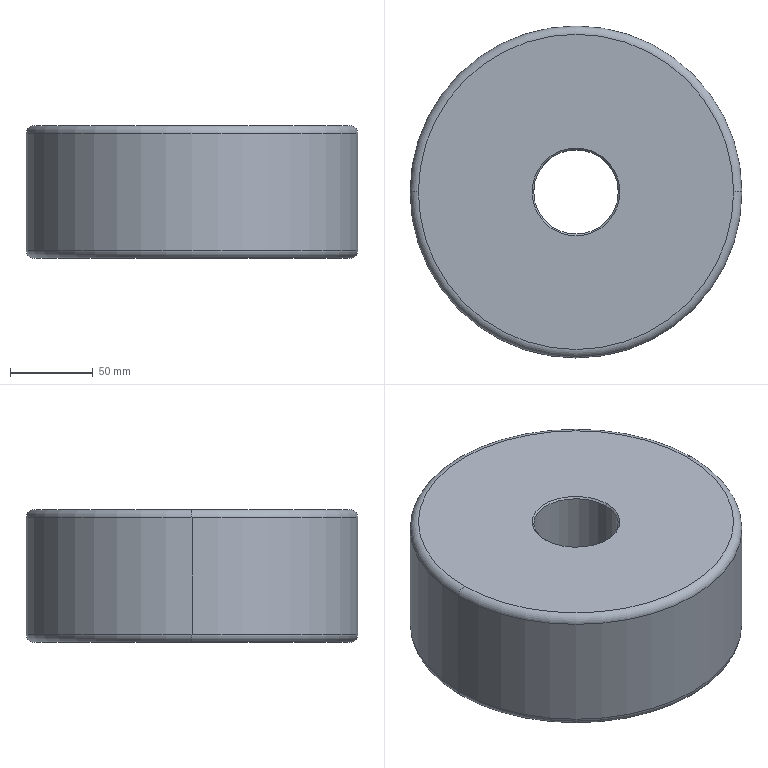Part | SolidWorks | features Chamfer 1, Extrusion 1, Fillet 1 | 1 solid | 14 faces | box 200 x 200 x 80 mm | volume 2343020 mm3 | cone 4 | torus 4 | cylinder 4 | plane 2 | commonest cylinder face diameters 51 x2 200 x2
STEP:
#1=CARTESIAN_POINT('',(25.5,0.,1.));
#2=VERTEX_POINT('',#1);
#3=CARTESIAN_POINT('',(-25.5,0.,1.));
#4=VERTEX_POINT('',#3);
#5=CARTESIAN_POINT('',(0.,0.,1.));
#6=DIRECTION('',(0.,0.,-1.));
#7=DIRECTION('',(1.,0.,0.));
#8=AXIS2_PLACEMENT_3D('',#5,#6,#7);
#9=CIRCLE('',#8,25.5);
#10=EDGE_CURVE('',#2,#4,#9,.T.);
#11=ORIENTED_EDGE('',*,*,#10,.F.);
#12=CARTESIAN_POINT('',(26.5,0.,0.));
#13=VERTEX_POINT('',#12);
#14=CARTESIAN_POINT('',(26.5,0.,0.));
#15=DIRECTION('',(0.7071,0.,-0.7071));
#16=VECTOR('',#15,1000.);
#17=LINE('',#14,#16);
#18=EDGE_CURVE('',#2,#13,#17,.T.);
#19=ORIENTED_EDGE('',*,*,#18,.T.);
#20=CARTESIAN_POINT('',(-26.5,0.,0.));
#21=VERTEX_POINT('',#20);
#22=CARTESIAN_POINT('',(0.,0.,0.));
#23=DIRECTION('',(0.,0.,1.));
#24=DIRECTION('',(1.,0.,0.));
#25=AXIS2_PLACEMENT_3D('',#22,#23,#24);
#26=CIRCLE('',#25,26.5);
#27=EDGE_CURVE('',#21,#13,#26,.T.);
#28=ORIENTED_EDGE('',*,*,#27,.F.);
#29=CARTESIAN_POINT('',(-26.5,0.,0.));
#30=DIRECTION('',(-0.7071,0.,-0.7071));
#31=VECTOR('',#30,1000.);
#32=LINE('',#29,#31);
#33=EDGE_CURVE('',#4,#21,#32,.T.);
#34=ORIENTED_EDGE('',*,*,#33,.F.);
#35=EDGE_LOOP('',(#11,#19,#28,#34));
#36=FACE_OUTER_BOUND('',#35,.T.);
#37=CARTESIAN_POINT('',(0.,0.,0.));
#38=DIRECTION('',(0.,0.,-1.));
#39=DIRECTION('',(-1.,0.,0.));
#40=AXIS2_PLACEMENT_3D('',#37,#38,#39);
#41=CONICAL_SURFACE('',#40,26.5,0.7854);
#42=ADVANCED_FACE('',(#36),#41,.F.);
#43=CARTESIAN_POINT('',(-25.5,0.,79.));
#44=VERTEX_POINT('',#43);
#45=CARTESIAN_POINT('',(25.5,0.,79.));
#46=VERTEX_POINT('',#45);
#47=CARTESIAN_POINT('',(0.,0.,79.));
#48=DIRECTION('',(0.,0.,1.));
#49=DIRECTION('',(1.,0.,0.));
#50=AXIS2_PLACEMENT_3D('',#47,#48,#49);
#51=CIRCLE('',#50,25.5);
#52=EDGE_CURVE('',#44,#46,#51,.T.);
#53=ORIENTED_EDGE('',*,*,#52,.F.);
#54=CARTESIAN_POINT('',(-26.5,0.,80.));
#55=VERTEX_POINT('',#54);
#56=CARTESIAN_POINT('',(-25.5,0.,79.));
#57=DIRECTION('',(-0.7071,0.,0.7071));
#58=VECTOR('',#57,1000.);
#59=LINE('',#56,#58);
#60=EDGE_CURVE('',#44,#55,#59,.T.);
#61=ORIENTED_EDGE('',*,*,#60,.T.);
#62=CARTESIAN_POINT('',(26.5,0.,80.));
#63=VERTEX_POINT('',#62);
#64=CARTESIAN_POINT('',(0.,0.,80.));
#65=DIRECTION('',(0.,0.,-1.));
#66=DIRECTION('',(1.,0.,0.));
#67=AXIS2_PLACEMENT_3D('',#64,#65,#66);
#68=CIRCLE('',#67,26.5);
#69=EDGE_CURVE('',#63,#55,#68,.T.);
#70=ORIENTED_EDGE('',*,*,#69,.F.);
#71=CARTESIAN_POINT('',(25.5,0.,79.));
#72=DIRECTION('',(0.7071,0.,0.7071));
#73=VECTOR('',#72,1000.);
#74=LINE('',#71,#73);
#75=EDGE_CURVE('',#46,#63,#74,.T.);
#76=ORIENTED_EDGE('',*,*,#75,.F.);
#77=EDGE_LOOP('',(#53,#61,#70,#76));
#78=FACE_OUTER_BOUND('',#77,.T.);
#79=CARTESIAN_POINT('',(0.,0.,79.));
#80=DIRECTION('',(0.,0.,1.));
#81=DIRECTION('',(1.,0.,0.));
#82=AXIS2_PLACEMENT_3D('',#79,#80,#81);
#83=CONICAL_SURFACE('',#82,25.5,0.7854);
#84=ADVANCED_FACE('',(#78),#83,.F.);
#85=CARTESIAN_POINT('',(-100.,0.,75.));
#86=VERTEX_POINT('',#85);
#87=CARTESIAN_POINT('',(100.,0.,75.));
#88=VERTEX_POINT('',#87);
#89=CARTESIAN_POINT('',(0.,0.,75.));
#90=DIRECTION('',(0.,0.,-1.));
#91=DIRECTION('',(1.,0.,0.));
#92=AXIS2_PLACEMENT_3D('',#89,#90,#91);
#93=CIRCLE('',#92,100.);
#94=EDGE_CURVE('',#86,#88,#93,.T.);
#95=ORIENTED_EDGE('',*,*,#94,.F.);
#96=CARTESIAN_POINT('',(-95.,0.,80.));
#97=VERTEX_POINT('',#96);
#98=CARTESIAN_POINT('',(-95.,0.,75.));
#99=DIRECTION('',(0.,1.,0.));
#100=DIRECTION('',(-1.,0.,0.));
#101=AXIS2_PLACEMENT_3D('',#98,#99,#100);
#102=CIRCLE('',#101,5.);
#103=EDGE_CURVE('',#86,#97,#102,.T.);
#104=ORIENTED_EDGE('',*,*,#103,.T.);
#105=CARTESIAN_POINT('',(95.,0.,80.));
#106=VERTEX_POINT('',#105);
#107=CARTESIAN_POINT('',(0.,0.,80.));
#108=DIRECTION('',(0.,0.,1.));
#109=DIRECTION('',(1.,0.,0.));
#110=AXIS2_PLACEMENT_3D('',#107,#108,#109);
#111=CIRCLE('',#110,95.);
#112=EDGE_CURVE('',#106,#97,#111,.T.);
#113=ORIENTED_EDGE('',*,*,#112,.F.);
#114=CARTESIAN_POINT('',(95.,0.,75.));
#115=DIRECTION('',(0.,-1.,0.));
#116=DIRECTION('',(0.,0.,-1.));
#117=AXIS2_PLACEMENT_3D('',#114,#115,#116);
#118=CIRCLE('',#117,5.);
#119=EDGE_CURVE('',#88,#106,#118,.T.);
#120=ORIENTED_EDGE('',*,*,#119,.F.);
#121=EDGE_LOOP('',(#95,#104,#113,#120));
#122=FACE_OUTER_BOUND('',#121,.T.);
#123=CARTESIAN_POINT('',(0.,0.,75.));
#124=DIRECTION('',(0.,0.,1.));
#125=DIRECTION('',(1.,0.,0.));
#126=AXIS2_PLACEMENT_3D('',#123,#124,#125);
#127=TOROIDAL_SURFACE('',#126,95.,5.);
#128=ADVANCED_FACE('',(#122),#127,.T.);
#129=CARTESIAN_POINT('',(-95.,0.,0.));
#130=VERTEX_POINT('',#129);
#131=CARTESIAN_POINT('',(95.,0.,0.));
#132=VERTEX_POINT('',#131);
#133=CARTESIAN_POINT('',(0.,0.,0.));
#134=DIRECTION('',(0.,0.,-1.));
#135=DIRECTION('',(1.,0.,0.));
#136=AXIS2_PLACEMENT_3D('',#133,#134,#135);
#137=CIRCLE('',#136,95.);
#138=EDGE_CURVE('',#130,#132,#137,.T.);
#139=ORIENTED_EDGE('',*,*,#138,.F.);
#140=CARTESIAN_POINT('',(-100.,0.,5.));
#141=VERTEX_POINT('',#140);
#142=CARTESIAN_POINT('',(-95.,0.,5.));
#143=DIRECTION('',(0.,1.,0.));
#144=DIRECTION('',(-1.,0.,0.));
#145=AXIS2_PLACEMENT_3D('',#142,#143,#144);
#146=CIRCLE('',#145,5.);
#147=EDGE_CURVE('',#130,#141,#146,.T.);
#148=ORIENTED_EDGE('',*,*,#147,.T.);
#149=CARTESIAN_POINT('',(100.,0.,5.));
#150=VERTEX_POINT('',#149);
#151=CARTESIAN_POINT('',(0.,0.,5.));
#152=DIRECTION('',(0.,0.,1.));
#153=DIRECTION('',(1.,0.,0.));
#154=AXIS2_PLACEMENT_3D('',#151,#152,#153);
#155=CIRCLE('',#154,100.);
#156=EDGE_CURVE('',#150,#141,#155,.T.);
#157=ORIENTED_EDGE('',*,*,#156,.F.);
#158=CARTESIAN_POINT('',(95.,0.,5.));
#159=DIRECTION('',(0.,-1.,0.));
#160=DIRECTION('',(0.,0.,-1.));
#161=AXIS2_PLACEMENT_3D('',#158,#159,#160);
#162=CIRCLE('',#161,5.);
#163=EDGE_CURVE('',#132,#150,#162,.T.);
#164=ORIENTED_EDGE('',*,*,#163,.F.);
#165=EDGE_LOOP('',(#139,#148,#157,#164));
#166=FACE_OUTER_BOUND('',#165,.T.);
#167=CARTESIAN_POINT('',(0.,0.,5.));
#168=DIRECTION('',(0.,0.,1.));
#169=DIRECTION('',(1.,0.,0.));
#170=AXIS2_PLACEMENT_3D('',#167,#168,#169);
#171=TOROIDAL_SURFACE('',#170,95.,5.);
#172=ADVANCED_FACE('',(#166),#171,.T.);
#173=ORIENTED_EDGE('',*,*,#52,.T.);
#174=CARTESIAN_POINT('',(25.5,0.,80.));
#175=DIRECTION('',(0.,0.,-1.));
#176=VECTOR('',#175,1000.);
#177=LINE('',#174,#176);
#178=EDGE_CURVE('',#46,#2,#177,.T.);
#179=ORIENTED_EDGE('',*,*,#178,.T.);
#180=ORIENTED_EDGE('',*,*,#10,.T.);
#181=CARTESIAN_POINT('',(-25.5,0.,80.));
#182=DIRECTION('',(0.,0.,-1.));
#183=VECTOR('',#182,1000.);
#184=LINE('',#181,#183);
#185=EDGE_CURVE('',#44,#4,#184,.T.);
#186=ORIENTED_EDGE('',*,*,#185,.F.);
#187=EDGE_LOOP('',(#173,#179,#180,#186));
#188=FACE_OUTER_BOUND('',#187,.T.);
#189=CARTESIAN_POINT('',(0.,0.,80.));
#190=DIRECTION('',(0.,0.,-1.));
#191=DIRECTION('',(-1.,0.,0.));
#192=AXIS2_PLACEMENT_3D('',#189,#190,#191);
#193=CYLINDRICAL_SURFACE('',#192,25.5);
#194=ADVANCED_FACE('',(#188),#193,.F.);
#195=ORIENTED_EDGE('',*,*,#94,.T.);
#196=CARTESIAN_POINT('',(100.,0.,80.));
#197=DIRECTION('',(0.,0.,-1.));
#198=VECTOR('',#197,1000.);
#199=LINE('',#196,#198);
#200=EDGE_CURVE('',#88,#150,#199,.T.);
#201=ORIENTED_EDGE('',*,*,#200,.T.);
#202=ORIENTED_EDGE('',*,*,#156,.T.);
#203=CARTESIAN_POINT('',(-100.,0.,80.));
#204=DIRECTION('',(0.,0.,-1.));
#205=VECTOR('',#204,1000.);
#206=LINE('',#203,#205);
#207=EDGE_CURVE('',#86,#141,#206,.T.);
#208=ORIENTED_EDGE('',*,*,#207,.F.);
#209=EDGE_LOOP('',(#195,#201,#202,#208));
#210=FACE_OUTER_BOUND('',#209,.T.);
#211=CARTESIAN_POINT('',(0.,0.,80.));
#212=DIRECTION('',(0.,0.,-1.));
#213=DIRECTION('',(-1.,0.,0.));
#214=AXIS2_PLACEMENT_3D('',#211,#212,#213);
#215=CYLINDRICAL_SURFACE('',#214,100.);
#216=ADVANCED_FACE('',(#210),#215,.T.);
#217=ORIENTED_EDGE('',*,*,#69,.T.);
#218=CARTESIAN_POINT('',(0.,0.,80.));
#219=DIRECTION('',(0.,0.,-1.));
#220=DIRECTION('',(1.,0.,0.));
#221=AXIS2_PLACEMENT_3D('',#218,#219,#220);
#222=CIRCLE('',#221,26.5);
#223=EDGE_CURVE('',#55,#63,#222,.T.);
#224=ORIENTED_EDGE('',*,*,#223,.T.);
#225=EDGE_LOOP('',(#217,#224));
#226=FACE_BOUND('',#225,.T.);
#227=ORIENTED_EDGE('',*,*,#112,.T.);
#228=CARTESIAN_POINT('',(0.,0.,80.));
#229=DIRECTION('',(0.,0.,1.));
#230=DIRECTION('',(1.,0.,0.));
#231=AXIS2_PLACEMENT_3D('',#228,#229,#230);
#232=CIRCLE('',#231,95.);
#233=EDGE_CURVE('',#97,#106,#232,.T.);
#234=ORIENTED_EDGE('',*,*,#233,.T.);
#235=EDGE_LOOP('',(#227,#234));
#236=FACE_OUTER_BOUND('',#235,.T.);
#237=CARTESIAN_POINT('',(0.,0.,80.));
#238=DIRECTION('',(0.,0.,1.));
#239=DIRECTION('',(1.,0.,0.));
#240=AXIS2_PLACEMENT_3D('',#237,#238,#239);
#241=PLANE('',#240);
#242=ADVANCED_FACE('',(#226,#236),#241,.T.);
#243=ORIENTED_EDGE('',*,*,#27,.T.);
#244=CARTESIAN_POINT('',(0.,0.,0.));
#245=DIRECTION('',(0.,0.,1.));
#246=DIRECTION('',(1.,0.,0.));
#247=AXIS2_PLACEMENT_3D('',#244,#245,#246);
#248=CIRCLE('',#247,26.5);
#249=EDGE_CURVE('',#13,#21,#248,.T.);
#250=ORIENTED_EDGE('',*,*,#249,.T.);
#251=EDGE_LOOP('',(#243,#250));
#252=FACE_BOUND('',#251,.T.);
#253=CARTESIAN_POINT('',(0.,0.,0.));
#254=DIRECTION('',(0.,0.,-1.));
#255=DIRECTION('',(1.,0.,0.));
#256=AXIS2_PLACEMENT_3D('',#253,#254,#255);
#257=CIRCLE('',#256,95.);
#258=EDGE_CURVE('',#132,#130,#257,.T.);
#259=ORIENTED_EDGE('',*,*,#258,.T.);
#260=ORIENTED_EDGE('',*,*,#138,.T.);
#261=EDGE_LOOP('',(#259,#260));
#262=FACE_OUTER_BOUND('',#261,.T.);
#263=CARTESIAN_POINT('',(0.,0.,0.));
#264=DIRECTION('',(0.,0.,1.));
#265=DIRECTION('',(1.,0.,0.));
#266=AXIS2_PLACEMENT_3D('',#263,#264,#265);
#267=PLANE('',#266);
#268=ADVANCED_FACE('',(#252,#262),#267,.F.);
#269=ORIENTED_EDGE('',*,*,#200,.F.);
#270=CARTESIAN_POINT('',(0.,0.,75.));
#271=DIRECTION('',(0.,0.,-1.));
#272=DIRECTION('',(1.,0.,0.));
#273=AXIS2_PLACEMENT_3D('',#270,#271,#272);
#274=CIRCLE('',#273,100.);
#275=EDGE_CURVE('',#88,#86,#274,.T.);
#276=ORIENTED_EDGE('',*,*,#275,.T.);
#277=ORIENTED_EDGE('',*,*,#207,.T.);
#278=CARTESIAN_POINT('',(0.,0.,5.));
#279=DIRECTION('',(0.,0.,1.));
#280=DIRECTION('',(1.,0.,0.));
#281=AXIS2_PLACEMENT_3D('',#278,#279,#280);
#282=CIRCLE('',#281,100.);
#283=EDGE_CURVE('',#141,#150,#282,.T.);
#284=ORIENTED_EDGE('',*,*,#283,.T.);
#285=EDGE_LOOP('',(#269,#276,#277,#284));
#286=FACE_OUTER_BOUND('',#285,.T.);
#287=CARTESIAN_POINT('',(0.,0.,80.));
#288=DIRECTION('',(0.,0.,-1.));
#289=DIRECTION('',(-1.,0.,0.));
#290=AXIS2_PLACEMENT_3D('',#287,#288,#289);
#291=CYLINDRICAL_SURFACE('',#290,100.);
#292=ADVANCED_FACE('',(#286),#291,.T.);
#293=ORIENTED_EDGE('',*,*,#178,.F.);
#294=CARTESIAN_POINT('',(0.,0.,79.));
#295=DIRECTION('',(0.,0.,1.));
#296=DIRECTION('',(1.,0.,0.));
#297=AXIS2_PLACEMENT_3D('',#294,#295,#296);
#298=CIRCLE('',#297,25.5);
#299=EDGE_CURVE('',#46,#44,#298,.T.);
#300=ORIENTED_EDGE('',*,*,#299,.T.);
#301=ORIENTED_EDGE('',*,*,#185,.T.);
#302=CARTESIAN_POINT('',(0.,0.,1.));
#303=DIRECTION('',(0.,0.,-1.));
#304=DIRECTION('',(1.,0.,0.));
#305=AXIS2_PLACEMENT_3D('',#302,#303,#304);
#306=CIRCLE('',#305,25.5);
#307=EDGE_CURVE('',#4,#2,#306,.T.);
#308=ORIENTED_EDGE('',*,*,#307,.T.);
#309=EDGE_LOOP('',(#293,#300,#301,#308));
#310=FACE_OUTER_BOUND('',#309,.T.);
#311=CARTESIAN_POINT('',(0.,0.,80.));
#312=DIRECTION('',(0.,0.,-1.));
#313=DIRECTION('',(-1.,0.,0.));
#314=AXIS2_PLACEMENT_3D('',#311,#312,#313);
#315=CYLINDRICAL_SURFACE('',#314,25.5);
#316=ADVANCED_FACE('',(#310),#315,.F.);
#317=ORIENTED_EDGE('',*,*,#147,.F.);
#318=ORIENTED_EDGE('',*,*,#258,.F.);
#319=ORIENTED_EDGE('',*,*,#163,.T.);
#320=ORIENTED_EDGE('',*,*,#283,.F.);
#321=EDGE_LOOP('',(#317,#318,#319,#320));
#322=FACE_OUTER_BOUND('',#321,.T.);
#323=CARTESIAN_POINT('',(0.,0.,5.));
#324=DIRECTION('',(0.,0.,1.));
#325=DIRECTION('',(1.,0.,0.));
#326=AXIS2_PLACEMENT_3D('',#323,#324,#325);
#327=TOROIDAL_SURFACE('',#326,95.,5.);
#328=ADVANCED_FACE('',(#322),#327,.T.);
#329=ORIENTED_EDGE('',*,*,#103,.F.);
#330=ORIENTED_EDGE('',*,*,#275,.F.);
#331=ORIENTED_EDGE('',*,*,#119,.T.);
#332=ORIENTED_EDGE('',*,*,#233,.F.);
#333=EDGE_LOOP('',(#329,#330,#331,#332));
#334=FACE_OUTER_BOUND('',#333,.T.);
#335=CARTESIAN_POINT('',(0.,0.,75.));
#336=DIRECTION('',(0.,0.,1.));
#337=DIRECTION('',(1.,0.,0.));
#338=AXIS2_PLACEMENT_3D('',#335,#336,#337);
#339=TOROIDAL_SURFACE('',#338,95.,5.);
#340=ADVANCED_FACE('',(#334),#339,.T.);
#341=ORIENTED_EDGE('',*,*,#60,.F.);
#342=ORIENTED_EDGE('',*,*,#299,.F.);
#343=ORIENTED_EDGE('',*,*,#75,.T.);
#344=ORIENTED_EDGE('',*,*,#223,.F.);
#345=EDGE_LOOP('',(#341,#342,#343,#344));
#346=FACE_OUTER_BOUND('',#345,.T.);
#347=CARTESIAN_POINT('',(0.,0.,79.));
#348=DIRECTION('',(0.,0.,1.));
#349=DIRECTION('',(1.,0.,0.));
#350=AXIS2_PLACEMENT_3D('',#347,#348,#349);
#351=CONICAL_SURFACE('',#350,25.5,0.7854);
#352=ADVANCED_FACE('',(#346),#351,.F.);
#353=ORIENTED_EDGE('',*,*,#18,.F.);
#354=ORIENTED_EDGE('',*,*,#307,.F.);
#355=ORIENTED_EDGE('',*,*,#33,.T.);
#356=ORIENTED_EDGE('',*,*,#249,.F.);
#357=EDGE_LOOP('',(#353,#354,#355,#356));
#358=FACE_OUTER_BOUND('',#357,.T.);
#359=CARTESIAN_POINT('',(0.,0.,0.));
#360=DIRECTION('',(0.,0.,-1.));
#361=DIRECTION('',(-1.,0.,0.));
#362=AXIS2_PLACEMENT_3D('',#359,#360,#361);
#363=CONICAL_SURFACE('',#362,26.5,0.7854);
#364=ADVANCED_FACE('',(#358),#363,.F.);
#365=CLOSED_SHELL('',(#42,#84,#128,#172,#194,#216,#242,#268,#292,#316,#328,#340,#352,#364));
#366=MANIFOLD_SOLID_BREP('',#365);
#367=CARTESIAN_POINT('',(0.,0.,0.));
#368=DIRECTION('',(0.,0.,1.));
#369=DIRECTION('',(1.,0.,0.));
#370=AXIS2_PLACEMENT_3D('',#367,#368,#369);
#371=(LENGTH_UNIT()NAMED_UNIT(*)SI_UNIT(.MILLI.,.METRE.));
#372=UNCERTAINTY_MEASURE_WITH_UNIT(LENGTH_MEASURE(0.00001),#371,'','');
#373=(NAMED_UNIT(*)PLANE_ANGLE_UNIT()SI_UNIT($,.RADIAN.));
#374=(NAMED_UNIT(*)SI_UNIT($,.STERADIAN.)SOLID_ANGLE_UNIT());
#375=(GEOMETRIC_REPRESENTATION_CONTEXT(3)GLOBAL_UNCERTAINTY_ASSIGNED_CONTEXT((#372))GLOBAL_UNIT_ASSIGNED_CONTEXT((#371,#373,#374))REPRESENTATION_CONTEXT('',''));
#376=ADVANCED_BREP_SHAPE_REPRESENTATION('',(#366,#370),#375);